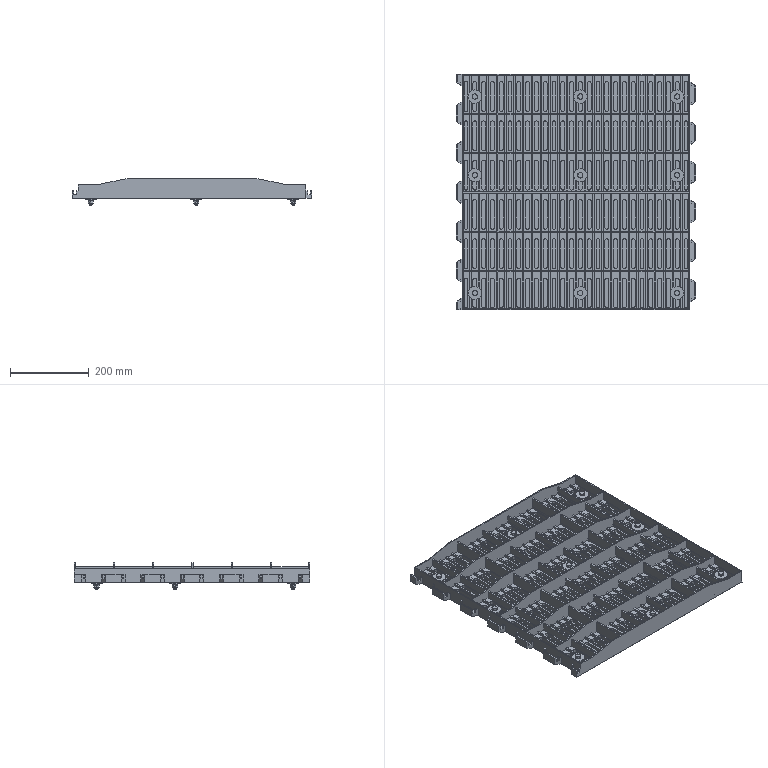Part | SolidWorks | features ReferencePattern 30, LocalLPattern 2 | 47 solids | 2236 faces | box 610 x 600 x 67 mm | volume 3647743 mm3 | plane 1478 | cylinder 524 | cone 216 | torus 18 | commonest cylinder face diameters 10 x330 8 x36 8.1 x27 12.277 x27 9 x18 11 x18